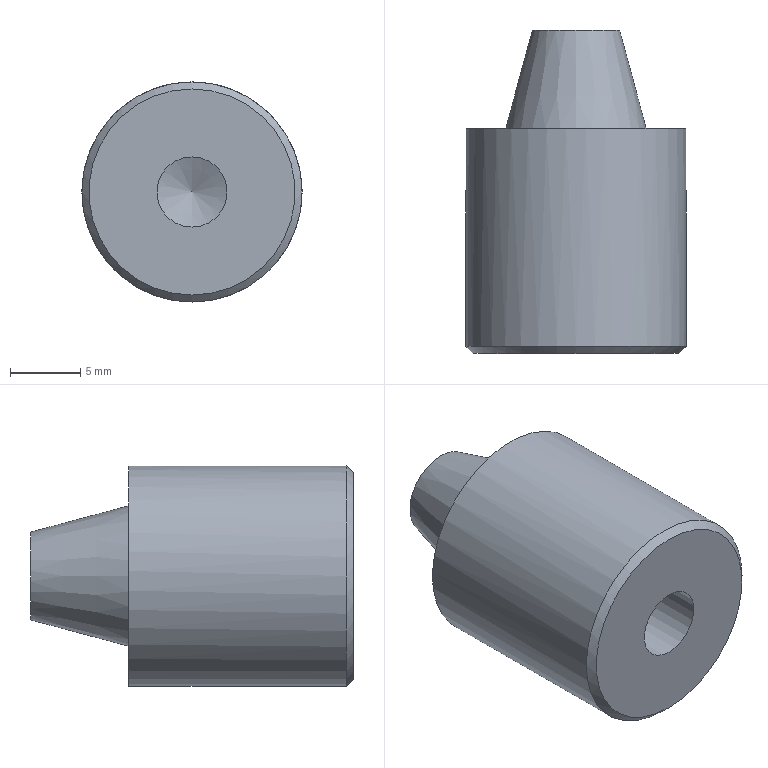Part | STEP file | Z05-16-1_id126_x_t | 1 solid | 8 faces | box 15.681 x 23 x 15.681 mm | volume 3250 mm3 | cone 3 | plane 3 | cylinder 2 | commonest cylinder face diameters 5 x1 15.681 x1
STEP:
#1=CARTESIAN_POINT('',(140.,-5.5,180.));
#2=VERTEX_POINT('',#1);
#3=VERTEX_LOOP('',#2);
#4=FACE_BOUND('',#3,.T.);
#5=CARTESIAN_POINT('',(140.,-6.5,177.5));
#6=VERTEX_POINT('',#5);
#7=CARTESIAN_POINT('',(140.,-6.5,180.));
#8=DIRECTION('',(0.,-1.,0.));
#9=DIRECTION('',(0.,0.,-1.));
#10=AXIS2_PLACEMENT_3D('',#7,#8,#9);
#11=CIRCLE('',#10,2.5);
#12=EDGE_CURVE('',#6,#6,#11,.T.);
#13=ORIENTED_EDGE('',*,*,#12,.T.);
#14=EDGE_LOOP('',(#13));
#15=FACE_BOUND('',#14,.T.);
#16=CARTESIAN_POINT('',(140.,-6.5,180.));
#17=DIRECTION('',(0.,-1.,0.));
#18=DIRECTION('',(0.,0.,-1.));
#19=AXIS2_PLACEMENT_3D('',#16,#17,#18);
#20=CONICAL_SURFACE('',#19,2.5,68.199);
#21=ADVANCED_FACE('',(#4,#15),#20,.F.);
#22=CARTESIAN_POINT('',(140.,6.5,176.876));
#23=VERTEX_POINT('',#22);
#24=CARTESIAN_POINT('',(140.,6.5,180.));
#25=DIRECTION('',(0.,-1.,0.));
#26=DIRECTION('',(0.,0.,-1.));
#27=AXIS2_PLACEMENT_3D('',#24,#25,#26);
#28=CIRCLE('',#27,3.124);
#29=EDGE_CURVE('',#23,#23,#28,.T.);
#30=ORIENTED_EDGE('',*,*,#29,.F.);
#31=EDGE_LOOP('',(#30));
#32=FACE_OUTER_BOUND('',#31,.T.);
#33=CARTESIAN_POINT('',(140.,6.5,180.));
#34=DIRECTION('',(0.,-1.,0.));
#35=DIRECTION('',(0.,0.,-1.));
#36=AXIS2_PLACEMENT_3D('',#33,#34,#35);
#37=PLANE('',#36);
#38=ADVANCED_FACE('',(#32),#37,.F.);
#39=ORIENTED_EDGE('',*,*,#12,.F.);
#40=EDGE_LOOP('',(#39));
#41=FACE_BOUND('',#40,.T.);
#42=CARTESIAN_POINT('',(140.,-16.5,177.5));
#43=VERTEX_POINT('',#42);
#44=CARTESIAN_POINT('',(140.,-16.5,180.));
#45=DIRECTION('',(0.,1.,0.));
#46=DIRECTION('',(0.,0.,-1.));
#47=AXIS2_PLACEMENT_3D('',#44,#45,#46);
#48=CIRCLE('',#47,2.5);
#49=EDGE_CURVE('',#43,#43,#48,.T.);
#50=ORIENTED_EDGE('',*,*,#49,.F.);
#51=EDGE_LOOP('',(#50));
#52=FACE_BOUND('',#51,.T.);
#53=CARTESIAN_POINT('',(140.,7.65,180.));
#54=DIRECTION('',(0.,-1.,0.));
#55=DIRECTION('',(0.,0.,-1.));
#56=AXIS2_PLACEMENT_3D('',#53,#54,#55);
#57=CYLINDRICAL_SURFACE('',#56,2.5);
#58=ADVANCED_FACE('',(#41,#52),#57,.F.);
#59=ORIENTED_EDGE('',*,*,#29,.T.);
#60=EDGE_LOOP('',(#59));
#61=FACE_BOUND('',#60,.T.);
#62=CARTESIAN_POINT('',(140.,-0.5,175.));
#63=VERTEX_POINT('',#62);
#64=CARTESIAN_POINT('',(140.,-0.5,180.));
#65=DIRECTION('',(0.,1.,0.));
#66=DIRECTION('',(0.,0.,-1.));
#67=AXIS2_PLACEMENT_3D('',#64,#65,#66);
#68=CIRCLE('',#67,5.);
#69=EDGE_CURVE('',#63,#63,#68,.T.);
#70=ORIENTED_EDGE('',*,*,#69,.T.);
#71=EDGE_LOOP('',(#70));
#72=FACE_BOUND('',#71,.T.);
#73=CARTESIAN_POINT('',(140.,-0.5,180.));
#74=DIRECTION('',(0.,-1.,0.));
#75=DIRECTION('',(0.,0.,-1.));
#76=AXIS2_PLACEMENT_3D('',#73,#74,#75);
#77=CONICAL_SURFACE('',#76,5.,15.);
#78=ADVANCED_FACE('',(#61,#72),#77,.T.);
#79=ORIENTED_EDGE('',*,*,#49,.T.);
#80=EDGE_LOOP('',(#79));
#81=FACE_BOUND('',#80,.T.);
#82=CARTESIAN_POINT('',(140.,-16.5,187.341));
#83=VERTEX_POINT('',#82);
#84=CARTESIAN_POINT('',(140.,-16.5,180.));
#85=DIRECTION('',(0.,1.,0.));
#86=DIRECTION('',(0.,0.,1.));
#87=AXIS2_PLACEMENT_3D('',#84,#85,#86);
#88=CIRCLE('',#87,7.341);
#89=EDGE_CURVE('',#83,#83,#88,.T.);
#90=ORIENTED_EDGE('',*,*,#89,.F.);
#91=EDGE_LOOP('',(#90));
#92=FACE_BOUND('',#91,.T.);
#93=CARTESIAN_POINT('',(140.,-16.5,180.));
#94=DIRECTION('',(0.,-1.,0.));
#95=DIRECTION('',(0.,0.,-1.));
#96=AXIS2_PLACEMENT_3D('',#93,#94,#95);
#97=PLANE('',#96);
#98=ADVANCED_FACE('',(#81,#92),#97,.T.);
#99=ORIENTED_EDGE('',*,*,#69,.F.);
#100=EDGE_LOOP('',(#99));
#101=FACE_BOUND('',#100,.T.);
#102=CARTESIAN_POINT('',(140.,-0.5,172.159));
#103=VERTEX_POINT('',#102);
#104=CARTESIAN_POINT('',(140.,-0.5,180.));
#105=DIRECTION('',(0.,-1.,0.));
#106=DIRECTION('',(0.,0.,-1.));
#107=AXIS2_PLACEMENT_3D('',#104,#105,#106);
#108=CIRCLE('',#107,7.841);
#109=EDGE_CURVE('',#103,#103,#108,.T.);
#110=ORIENTED_EDGE('',*,*,#109,.F.);
#111=EDGE_LOOP('',(#110));
#112=FACE_BOUND('',#111,.T.);
#113=CARTESIAN_POINT('',(140.,-0.5,180.));
#114=DIRECTION('',(0.,-1.,0.));
#115=DIRECTION('',(0.,0.,-1.));
#116=AXIS2_PLACEMENT_3D('',#113,#114,#115);
#117=PLANE('',#116);
#118=ADVANCED_FACE('',(#101,#112),#117,.F.);
#119=ORIENTED_EDGE('',*,*,#89,.T.);
#120=EDGE_LOOP('',(#119));
#121=FACE_BOUND('',#120,.T.);
#122=CARTESIAN_POINT('',(140.,-16.,172.159));
#123=VERTEX_POINT('',#122);
#124=CARTESIAN_POINT('',(140.,-16.,180.));
#125=DIRECTION('',(0.,1.,0.));
#126=DIRECTION('',(0.,0.,-1.));
#127=AXIS2_PLACEMENT_3D('',#124,#125,#126);
#128=CIRCLE('',#127,7.841);
#129=EDGE_CURVE('',#123,#123,#128,.T.);
#130=ORIENTED_EDGE('',*,*,#129,.F.);
#131=EDGE_LOOP('',(#130));
#132=FACE_BOUND('',#131,.T.);
#133=CARTESIAN_POINT('',(140.,-16.,180.));
#134=DIRECTION('',(0.,1.,0.));
#135=DIRECTION('',(0.,0.,1.));
#136=AXIS2_PLACEMENT_3D('',#133,#134,#135);
#137=CONICAL_SURFACE('',#136,7.841,45.);
#138=ADVANCED_FACE('',(#121,#132),#137,.T.);
#139=ORIENTED_EDGE('',*,*,#129,.T.);
#140=EDGE_LOOP('',(#139));
#141=FACE_BOUND('',#140,.T.);
#142=ORIENTED_EDGE('',*,*,#109,.T.);
#143=EDGE_LOOP('',(#142));
#144=FACE_BOUND('',#143,.T.);
#145=CARTESIAN_POINT('',(140.,7.65,180.));
#146=DIRECTION('',(0.,-1.,0.));
#147=DIRECTION('',(0.,0.,-1.));
#148=AXIS2_PLACEMENT_3D('',#145,#146,#147);
#149=CYLINDRICAL_SURFACE('',#148,7.841);
#150=ADVANCED_FACE('',(#141,#144),#149,.T.);
#151=CLOSED_SHELL('',(#21,#38,#58,#78,#98,#118,#138,#150));
#152=MANIFOLD_SOLID_BREP('',#151);
#153=(LENGTH_UNIT()NAMED_UNIT(*)SI_UNIT(.MILLI.,.METRE.));
#154=UNCERTAINTY_MEASURE_WITH_UNIT(LENGTH_MEASURE(0.00004123),#153,'','');
#155=(NAMED_UNIT(*)PLANE_ANGLE_UNIT()SI_UNIT($,.RADIAN.));
#156=PLANE_ANGLE_MEASURE_WITH_UNIT(PLANE_ANGLE_MEASURE(0.01745),#155);
#157=DIMENSIONAL_EXPONENTS(0.,0.,0.,0.,0.,0.,0.);
#158=(CONVERSION_BASED_UNIT('DEGREE',#156)NAMED_UNIT(#157)PLANE_ANGLE_UNIT());
#159=(NAMED_UNIT(*)SI_UNIT($,.STERADIAN.)SOLID_ANGLE_UNIT());
#160=(GEOMETRIC_REPRESENTATION_CONTEXT(3)GLOBAL_UNCERTAINTY_ASSIGNED_CONTEXT((#154))GLOBAL_UNIT_ASSIGNED_CONTEXT((#153,#158,#159))REPRESENTATION_CONTEXT('',''));
#161=ADVANCED_BREP_SHAPE_REPRESENTATION('',(#152),#160);